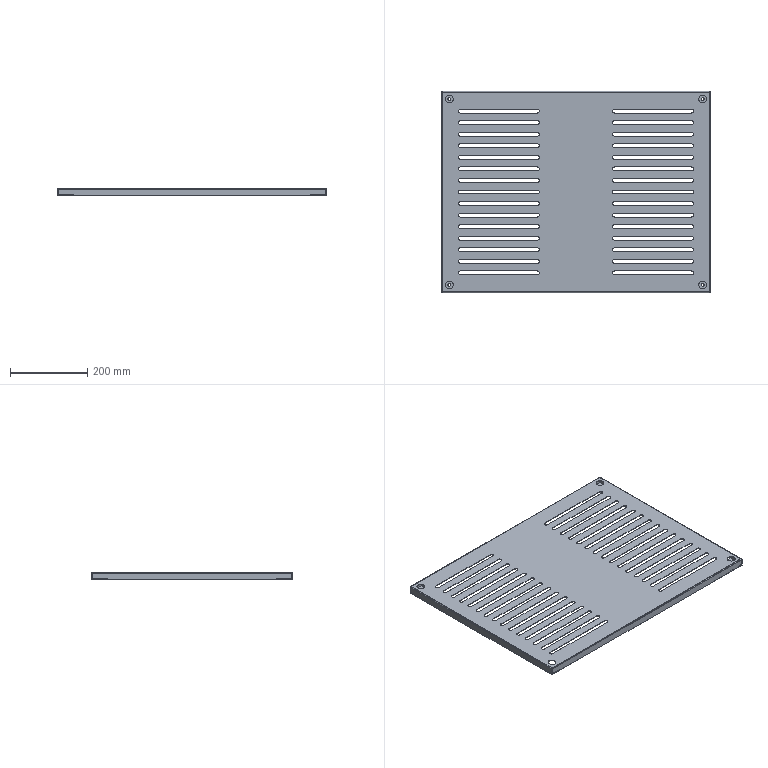Part | STEP file | Box sheet metal_default<machined> | 5 solids | 260 faces | box 698 x 522 x 20 mm | volume 532626 mm3 | plane 122 | cylinder 118 | spline 20 | commonest cylinder face diameters 10 x90 7 x8 20 x8 1.5 x4 2 x4 4.5 x4